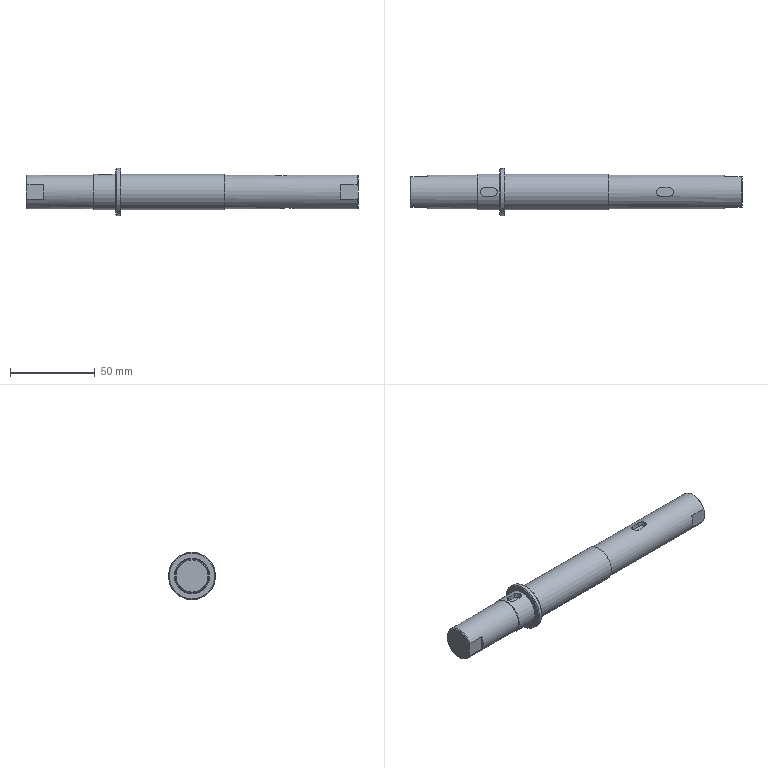Part | NX | features BREP 1 | 1 solid | 43 faces | box 196 x 28 x 28 mm | volume 62604 mm3 | plane 23 | cylinder 13 | cone 7 | commonest cylinder face diameters 5 x4 6.8 x4 20 x2 21 x2 28 x1
STEP:
#1=CARTESIAN_POINT('',(55.5,0.,14.));
#2=VERTEX_POINT('',#1);
#3=CARTESIAN_POINT('',(55.5,0.,0.));
#4=DIRECTION('',(-1.,0.,0.));
#5=DIRECTION('',(0.,0.,1.));
#6=AXIS2_PLACEMENT_3D('',#3,#4,#5);
#7=CIRCLE('',#6,14.);
#8=EDGE_CURVE('',#2,#2,#7,.T.);
#9=ORIENTED_EDGE('',*,*,#8,.F.);
#10=EDGE_LOOP('',(#9));
#11=FACE_BOUND('',#10,.T.);
#12=CARTESIAN_POINT('',(56.,0.,13.5));
#13=VERTEX_POINT('',#12);
#14=CARTESIAN_POINT('',(56.,0.,0.));
#15=DIRECTION('',(1.,0.,0.));
#16=DIRECTION('',(0.,0.,1.));
#17=AXIS2_PLACEMENT_3D('',#14,#15,#16);
#18=CIRCLE('',#17,13.5);
#19=EDGE_CURVE('',#13,#13,#18,.T.);
#20=ORIENTED_EDGE('',*,*,#19,.F.);
#21=EDGE_LOOP('',(#20));
#22=FACE_BOUND('',#21,.T.);
#23=CARTESIAN_POINT('',(55.5,0.,0.));
#24=DIRECTION('',(-1.,0.,0.));
#25=DIRECTION('',(0.,0.,1.));
#26=AXIS2_PLACEMENT_3D('',#23,#24,#25);
#27=CONICAL_SURFACE('',#26,14.,0.7854);
#28=ADVANCED_FACE('',(#11,#22),#27,.T.);
#29=CARTESIAN_POINT('',(53.5,0.,-14.));
#30=VERTEX_POINT('',#29);
#31=CARTESIAN_POINT('',(53.5,0.,0.));
#32=DIRECTION('',(1.,0.,0.));
#33=DIRECTION('',(0.,0.,-1.));
#34=AXIS2_PLACEMENT_3D('',#31,#32,#33);
#35=CIRCLE('',#34,14.);
#36=EDGE_CURVE('',#30,#30,#35,.T.);
#37=ORIENTED_EDGE('',*,*,#36,.F.);
#38=EDGE_LOOP('',(#37));
#39=FACE_BOUND('',#38,.T.);
#40=CARTESIAN_POINT('',(53.,0.,-13.5));
#41=VERTEX_POINT('',#40);
#42=CARTESIAN_POINT('',(53.,0.,0.));
#43=DIRECTION('',(-1.,0.,0.));
#44=DIRECTION('',(0.,0.,-1.));
#45=AXIS2_PLACEMENT_3D('',#42,#43,#44);
#46=CIRCLE('',#45,13.5);
#47=EDGE_CURVE('',#41,#41,#46,.T.);
#48=ORIENTED_EDGE('',*,*,#47,.F.);
#49=EDGE_LOOP('',(#48));
#50=FACE_BOUND('',#49,.T.);
#51=CARTESIAN_POINT('',(53.,0.,0.));
#52=DIRECTION('',(1.,0.,0.));
#53=DIRECTION('',(0.,0.,-1.));
#54=AXIS2_PLACEMENT_3D('',#51,#52,#53);
#55=CONICAL_SURFACE('',#54,13.5,0.7854);
#56=ADVANCED_FACE('',(#39,#50),#55,.T.);
#57=CARTESIAN_POINT('',(196.,0.,5.4));
#58=VERTEX_POINT('',#57);
#59=CARTESIAN_POINT('',(196.,0.,0.));
#60=DIRECTION('',(-1.,0.,0.));
#61=DIRECTION('',(0.,0.,1.));
#62=AXIS2_PLACEMENT_3D('',#59,#60,#61);
#63=CIRCLE('',#62,5.4);
#64=EDGE_CURVE('',#58,#58,#63,.T.);
#65=ORIENTED_EDGE('',*,*,#64,.F.);
#66=EDGE_LOOP('',(#65));
#67=FACE_BOUND('',#66,.T.);
#68=CARTESIAN_POINT('',(194.,0.,3.4));
#69=VERTEX_POINT('',#68);
#70=CARTESIAN_POINT('',(194.,0.,0.));
#71=DIRECTION('',(1.,0.,0.));
#72=DIRECTION('',(0.,0.,1.));
#73=AXIS2_PLACEMENT_3D('',#70,#71,#72);
#74=CIRCLE('',#73,3.4);
#75=EDGE_CURVE('',#69,#69,#74,.T.);
#76=ORIENTED_EDGE('',*,*,#75,.F.);
#77=EDGE_LOOP('',(#76));
#78=FACE_BOUND('',#77,.T.);
#79=CARTESIAN_POINT('',(194.,0.,0.));
#80=DIRECTION('',(1.,0.,0.));
#81=DIRECTION('',(0.,0.,-1.));
#82=AXIS2_PLACEMENT_3D('',#79,#80,#81);
#83=CONICAL_SURFACE('',#82,3.4,0.7854);
#84=ADVANCED_FACE('',(#67,#78),#83,.F.);
#85=CARTESIAN_POINT('',(196.,9.,3.041));
#86=VERTEX_POINT('',#85);
#87=CARTESIAN_POINT('',(196.,-9.,3.041));
#88=VERTEX_POINT('',#87);
#89=CARTESIAN_POINT('',(196.,0.,0.));
#90=DIRECTION('',(1.,0.,0.));
#91=DIRECTION('',(0.,0.,1.));
#92=AXIS2_PLACEMENT_3D('',#89,#90,#91);
#93=CIRCLE('',#92,9.5);
#94=EDGE_CURVE('',#86,#88,#93,.T.);
#95=ORIENTED_EDGE('',*,*,#94,.F.);
#96=CARTESIAN_POINT('',(195.5,9.,4.359));
#97=VERTEX_POINT('',#96);
#98=CARTESIAN_POINT('',(195.5,9.,4.359));
#99=CARTESIAN_POINT('',(195.688,9.,3.928));
#100=CARTESIAN_POINT('',(195.857,9.,3.489));
#101=CARTESIAN_POINT('',(196.,9.,3.041));
#102=B_SPLINE_CURVE_WITH_KNOTS('',3,(#98,#99,#100,#101),.UNSPECIFIED.,.F.,.F.,(4,4),(0.,1.),.PIECEWISE_BEZIER_KNOTS.);
#103=EDGE_CURVE('',#97,#86,#102,.T.);
#104=ORIENTED_EDGE('',*,*,#103,.F.);
#105=CARTESIAN_POINT('',(195.5,-9.,4.359));
#106=VERTEX_POINT('',#105);
#107=CARTESIAN_POINT('',(195.5,0.,0.));
#108=DIRECTION('',(-1.,0.,0.));
#109=DIRECTION('',(0.,0.,1.));
#110=AXIS2_PLACEMENT_3D('',#107,#108,#109);
#111=CIRCLE('',#110,10.);
#112=EDGE_CURVE('',#106,#97,#111,.T.);
#113=ORIENTED_EDGE('',*,*,#112,.F.);
#114=CARTESIAN_POINT('',(196.,-9.,3.041));
#115=CARTESIAN_POINT('',(195.857,-9.,3.489));
#116=CARTESIAN_POINT('',(195.688,-9.,3.928));
#117=CARTESIAN_POINT('',(195.5,-9.,4.359));
#118=B_SPLINE_CURVE_WITH_KNOTS('',3,(#114,#115,#116,#117),.UNSPECIFIED.,.F.,.F.,(4,4),(0.,1.),.PIECEWISE_BEZIER_KNOTS.);
#119=EDGE_CURVE('',#88,#106,#118,.T.);
#120=ORIENTED_EDGE('',*,*,#119,.F.);
#121=EDGE_LOOP('',(#95,#104,#113,#120));
#122=FACE_BOUND('',#121,.T.);
#123=CARTESIAN_POINT('',(195.5,0.,0.));
#124=DIRECTION('',(-1.,0.,0.));
#125=DIRECTION('',(0.,0.,1.));
#126=AXIS2_PLACEMENT_3D('',#123,#124,#125);
#127=CONICAL_SURFACE('',#126,10.,0.7854);
#128=ADVANCED_FACE('',(#122),#127,.T.);
#129=CARTESIAN_POINT('',(0.,9.,-3.041));
#130=VERTEX_POINT('',#129);
#131=CARTESIAN_POINT('',(0.,-9.,-3.041));
#132=VERTEX_POINT('',#131);
#133=CARTESIAN_POINT('',(0.,0.,0.));
#134=DIRECTION('',(-1.,0.,0.));
#135=DIRECTION('',(0.,0.,-1.));
#136=AXIS2_PLACEMENT_3D('',#133,#134,#135);
#137=CIRCLE('',#136,9.5);
#138=EDGE_CURVE('',#130,#132,#137,.T.);
#139=ORIENTED_EDGE('',*,*,#138,.F.);
#140=CARTESIAN_POINT('',(0.5,9.,-4.359));
#141=VERTEX_POINT('',#140);
#142=CARTESIAN_POINT('',(0.5,9.,-4.359));
#143=CARTESIAN_POINT('',(0.3123,9.,-3.928));
#144=CARTESIAN_POINT('',(0.1432,9.,-3.489));
#145=CARTESIAN_POINT('',(0.,9.,-3.041));
#146=B_SPLINE_CURVE_WITH_KNOTS('',3,(#142,#143,#144,#145),.UNSPECIFIED.,.F.,.F.,(4,4),(0.,1.),.PIECEWISE_BEZIER_KNOTS.);
#147=EDGE_CURVE('',#141,#130,#146,.T.);
#148=ORIENTED_EDGE('',*,*,#147,.F.);
#149=CARTESIAN_POINT('',(0.5,-9.,-4.359));
#150=VERTEX_POINT('',#149);
#151=CARTESIAN_POINT('',(0.5,0.,0.));
#152=DIRECTION('',(1.,0.,0.));
#153=DIRECTION('',(0.,0.,-1.));
#154=AXIS2_PLACEMENT_3D('',#151,#152,#153);
#155=CIRCLE('',#154,10.);
#156=EDGE_CURVE('',#150,#141,#155,.T.);
#157=ORIENTED_EDGE('',*,*,#156,.F.);
#158=CARTESIAN_POINT('',(0.,-9.,-3.041));
#159=CARTESIAN_POINT('',(0.1432,-9.,-3.489));
#160=CARTESIAN_POINT('',(0.3123,-9.,-3.928));
#161=CARTESIAN_POINT('',(0.5,-9.,-4.359));
#162=B_SPLINE_CURVE_WITH_KNOTS('',3,(#158,#159,#160,#161),.UNSPECIFIED.,.F.,.F.,(4,4),(0.,1.),.PIECEWISE_BEZIER_KNOTS.);
#163=EDGE_CURVE('',#132,#150,#162,.T.);
#164=ORIENTED_EDGE('',*,*,#163,.F.);
#165=EDGE_LOOP('',(#139,#148,#157,#164));
#166=FACE_BOUND('',#165,.T.);
#167=CARTESIAN_POINT('',(0.,0.,0.));
#168=DIRECTION('',(1.,0.,0.));
#169=DIRECTION('',(0.,0.,-1.));
#170=AXIS2_PLACEMENT_3D('',#167,#168,#169);
#171=CONICAL_SURFACE('',#170,9.5,0.7854);
#172=ADVANCED_FACE('',(#166),#171,.T.);
#173=CARTESIAN_POINT('',(117.,0.,-10.));
#174=VERTEX_POINT('',#173);
#175=CARTESIAN_POINT('',(117.,0.,0.));
#176=DIRECTION('',(1.,0.,0.));
#177=DIRECTION('',(0.,0.,-1.));
#178=AXIS2_PLACEMENT_3D('',#175,#176,#177);
#179=CIRCLE('',#178,10.);
#180=EDGE_CURVE('',#174,#174,#179,.T.);
#181=ORIENTED_EDGE('',*,*,#180,.T.);
#182=EDGE_LOOP('',(#181));
#183=FACE_BOUND('',#182,.T.);
#184=CARTESIAN_POINT('',(153.,-2.5,9.682));
#185=VERTEX_POINT('',#184);
#186=CARTESIAN_POINT('',(153.,2.5,9.682));
#187=VERTEX_POINT('',#186);
#188=CARTESIAN_POINT('',(153.,-2.5,9.682));
#189=CARTESIAN_POINT('',(153.663,-2.5,9.682));
#190=CARTESIAN_POINT('',(154.954,-1.958,9.844));
#191=CARTESIAN_POINT('',(155.773,-0.003505,10.078));
#192=CARTESIAN_POINT('',(154.955,1.959,9.844));
#193=CARTESIAN_POINT('',(153.663,2.5,9.682));
#194=CARTESIAN_POINT('',(153.,2.5,9.682));
#195=B_SPLINE_CURVE_WITH_KNOTS('',3,(#188,#189,#190,#191,#192,#193,#194),.UNSPECIFIED.,.F.,.F.,(4,1,1,1,4),(0.,0.001961,0.003922,0.005884,0.007845),.UNSPECIFIED.);
#196=EDGE_CURVE('',#185,#187,#195,.T.);
#197=ORIENTED_EDGE('',*,*,#196,.F.);
#198=CARTESIAN_POINT('',(148.,-2.5,9.682));
#199=VERTEX_POINT('',#198);
#200=CARTESIAN_POINT('',(0.,-2.5,9.682));
#201=DIRECTION('',(-1.,0.,0.));
#202=VECTOR('',#201,1000.);
#203=LINE('',#200,#202);
#204=EDGE_CURVE('',#185,#199,#203,.T.);
#205=ORIENTED_EDGE('',*,*,#204,.T.);
#206=CARTESIAN_POINT('',(148.,2.5,9.682));
#207=VERTEX_POINT('',#206);
#208=CARTESIAN_POINT('',(148.,-2.5,9.682));
#209=CARTESIAN_POINT('',(147.337,-2.5,9.682));
#210=CARTESIAN_POINT('',(146.046,-1.958,9.844));
#211=CARTESIAN_POINT('',(145.227,-0.003505,10.078));
#212=CARTESIAN_POINT('',(146.045,1.959,9.844));
#213=CARTESIAN_POINT('',(147.337,2.5,9.682));
#214=CARTESIAN_POINT('',(148.,2.5,9.682));
#215=B_SPLINE_CURVE_WITH_KNOTS('',3,(#208,#209,#210,#211,#212,#213,#214),.UNSPECIFIED.,.F.,.F.,(4,1,1,1,4),(0.,0.001961,0.003922,0.005884,0.007845),.UNSPECIFIED.);
#216=EDGE_CURVE('',#199,#207,#215,.T.);
#217=ORIENTED_EDGE('',*,*,#216,.T.);
#218=CARTESIAN_POINT('',(0.,2.5,9.682));
#219=DIRECTION('',(-1.,0.,0.));
#220=VECTOR('',#219,1000.);
#221=LINE('',#218,#220);
#222=EDGE_CURVE('',#187,#207,#221,.T.);
#223=ORIENTED_EDGE('',*,*,#222,.F.);
#224=EDGE_LOOP('',(#197,#205,#217,#223));
#225=FACE_BOUND('',#224,.T.);
#226=ORIENTED_EDGE('',*,*,#112,.T.);
#227=CARTESIAN_POINT('',(185.5,9.,4.359));
#228=VERTEX_POINT('',#227);
#229=CARTESIAN_POINT('',(185.5,9.,4.359));
#230=DIRECTION('',(1.,0.,0.));
#231=VECTOR('',#230,1000.);
#232=LINE('',#229,#231);
#233=EDGE_CURVE('',#228,#97,#232,.T.);
#234=ORIENTED_EDGE('',*,*,#233,.F.);
#235=CARTESIAN_POINT('',(185.5,9.,-4.359));
#236=VERTEX_POINT('',#235);
#237=CARTESIAN_POINT('',(185.5,0.,0.));
#238=DIRECTION('',(1.,0.,0.));
#239=DIRECTION('',(0.,0.,-1.));
#240=AXIS2_PLACEMENT_3D('',#237,#238,#239);
#241=CIRCLE('',#240,10.);
#242=EDGE_CURVE('',#236,#228,#241,.T.);
#243=ORIENTED_EDGE('',*,*,#242,.F.);
#244=CARTESIAN_POINT('',(195.5,9.,-4.359));
#245=VERTEX_POINT('',#244);
#246=CARTESIAN_POINT('',(185.5,9.,-4.359));
#247=DIRECTION('',(1.,0.,0.));
#248=VECTOR('',#247,1000.);
#249=LINE('',#246,#248);
#250=EDGE_CURVE('',#236,#245,#249,.T.);
#251=ORIENTED_EDGE('',*,*,#250,.T.);
#252=CARTESIAN_POINT('',(195.5,-9.,-4.359));
#253=VERTEX_POINT('',#252);
#254=CARTESIAN_POINT('',(195.5,0.,0.));
#255=DIRECTION('',(-1.,0.,0.));
#256=DIRECTION('',(0.,0.,1.));
#257=AXIS2_PLACEMENT_3D('',#254,#255,#256);
#258=CIRCLE('',#257,10.);
#259=EDGE_CURVE('',#245,#253,#258,.T.);
#260=ORIENTED_EDGE('',*,*,#259,.T.);
#261=CARTESIAN_POINT('',(185.5,-9.,-4.359));
#262=VERTEX_POINT('',#261);
#263=CARTESIAN_POINT('',(185.5,-9.,-4.359));
#264=DIRECTION('',(1.,0.,0.));
#265=VECTOR('',#264,1000.);
#266=LINE('',#263,#265);
#267=EDGE_CURVE('',#253,#262,#266,.F.);
#268=ORIENTED_EDGE('',*,*,#267,.T.);
#269=CARTESIAN_POINT('',(185.5,-9.,4.359));
#270=VERTEX_POINT('',#269);
#271=CARTESIAN_POINT('',(185.5,0.,0.));
#272=DIRECTION('',(1.,0.,0.));
#273=DIRECTION('',(0.,0.,-1.));
#274=AXIS2_PLACEMENT_3D('',#271,#272,#273);
#275=CIRCLE('',#274,10.);
#276=EDGE_CURVE('',#270,#262,#275,.T.);
#277=ORIENTED_EDGE('',*,*,#276,.F.);
#278=CARTESIAN_POINT('',(185.5,-9.,4.359));
#279=DIRECTION('',(1.,0.,0.));
#280=VECTOR('',#279,1000.);
#281=LINE('',#278,#280);
#282=EDGE_CURVE('',#106,#270,#281,.F.);
#283=ORIENTED_EDGE('',*,*,#282,.F.);
#284=EDGE_LOOP('',(#226,#234,#243,#251,#260,#268,#277,#283));
#285=FACE_BOUND('',#284,.T.);
#286=CARTESIAN_POINT('',(149.192,0.,-10.));
#287=VERTEX_POINT('',#286);
#288=CARTESIAN_POINT('',(149.694,-1.596,-9.901));
#289=CARTESIAN_POINT('',(148.941,0.0002752,-10.05));
#290=CARTESIAN_POINT('',(149.693,1.595,-9.901));
#291=CARTESIAN_POINT('',(151.021,2.554,-9.677));
#292=CARTESIAN_POINT('',(152.529,3.162,-9.492));
#293=CARTESIAN_POINT('',(154.665,3.539,-9.349));
#294=CARTESIAN_POINT('',(156.939,3.204,-9.507));
#295=CARTESIAN_POINT('',(158.514,1.646,-9.901));
#296=CARTESIAN_POINT('',(158.953,0.0115,-10.049));
#297=CARTESIAN_POINT('',(158.524,-1.631,-9.904));
#298=CARTESIAN_POINT('',(156.947,-3.202,-9.508));
#299=CARTESIAN_POINT('',(154.68,-3.539,-9.348));
#300=CARTESIAN_POINT('',(152.535,-3.164,-9.491));
#301=CARTESIAN_POINT('',(151.021,-2.554,-9.677));
#302=CARTESIAN_POINT('',(149.694,-1.596,-9.901));
#303=CARTESIAN_POINT('',(148.941,0.0002752,-10.05));
#304=CARTESIAN_POINT('',(149.693,1.595,-9.901));
#305=B_SPLINE_CURVE_WITH_KNOTS('',3,(#288,#289,#290,#291,#292,#293,#294,#295,#296,#297,#298,#299,#300,#301,#302,#303,#304),.UNSPECIFIED.,.T.,.F.,(1,1,1,1,1,1,1,1,1,1,1,1,1,1,1,1,1,1,1,1,1),(-0.004908,-0.003272,-0.001636,0.,0.001636,0.003272,0.004908,0.006544,0.009815,0.01145,0.01309,0.01472,0.01636,0.01963,0.02127,0.0229,0.02454,0.02617,0.02781,0.02945,0.03108),.UNSPECIFIED.);
#306=EDGE_CURVE('',#287,#287,#305,.T.);
#307=ORIENTED_EDGE('',*,*,#306,.F.);
#308=EDGE_LOOP('',(#307));
#309=FACE_BOUND('',#308,.T.);
#310=CARTESIAN_POINT('',(0.,0.,0.));
#311=DIRECTION('',(-1.,0.,0.));
#312=DIRECTION('',(0.,0.,1.));
#313=AXIS2_PLACEMENT_3D('',#310,#311,#312);
#314=CYLINDRICAL_SURFACE('',#313,10.);
#315=ADVANCED_FACE('',(#183,#225,#285,#309),#314,.T.);
#316=ORIENTED_EDGE('',*,*,#306,.T.);
#317=EDGE_LOOP('',(#316));
#318=FACE_BOUND('',#317,.T.);
#319=CARTESIAN_POINT('',(164.,-3.4,0.));
#320=VERTEX_POINT('',#319);
#321=CARTESIAN_POINT('',(165.408,0.,-3.4));
#322=VERTEX_POINT('',#321);
#323=CARTESIAN_POINT('',(164.,-3.4,0.));
#324=CARTESIAN_POINT('',(164.825,-3.4,-1.992));
#325=CARTESIAN_POINT('',(165.408,-1.992,-3.4));
#326=CARTESIAN_POINT('',(165.408,0.,-3.4));
#327=(BOUNDED_CURVE()B_SPLINE_CURVE(3,(#323,#324,#325,#326),.UNSPECIFIED.,.F.,.F.)B_SPLINE_CURVE_WITH_KNOTS((4,4),(0.,1.),.PIECEWISE_BEZIER_KNOTS.)CURVE()GEOMETRIC_REPRESENTATION_ITEM()RATIONAL_B_SPLINE_CURVE((1.,0.8047,0.8047,1.))REPRESENTATION_ITEM(''));
#328=EDGE_CURVE('',#320,#322,#327,.T.);
#329=ORIENTED_EDGE('',*,*,#328,.T.);
#330=CARTESIAN_POINT('',(164.,3.4,0.));
#331=VERTEX_POINT('',#330);
#332=CARTESIAN_POINT('',(165.408,0.,-3.4));
#333=CARTESIAN_POINT('',(165.408,1.992,-3.4));
#334=CARTESIAN_POINT('',(164.825,3.4,-1.992));
#335=CARTESIAN_POINT('',(164.,3.4,0.));
#336=(BOUNDED_CURVE()B_SPLINE_CURVE(3,(#332,#333,#334,#335),.UNSPECIFIED.,.F.,.F.)B_SPLINE_CURVE_WITH_KNOTS((4,4),(0.,1.),.PIECEWISE_BEZIER_KNOTS.)CURVE()GEOMETRIC_REPRESENTATION_ITEM()RATIONAL_B_SPLINE_CURVE((1.,0.8047,0.8047,1.))REPRESENTATION_ITEM(''));
#337=EDGE_CURVE('',#322,#331,#336,.T.);
#338=ORIENTED_EDGE('',*,*,#337,.T.);
#339=CARTESIAN_POINT('',(163.,3.375,-0.4142));
#340=VERTEX_POINT('',#339);
#341=CARTESIAN_POINT('',(164.,3.4,0.));
#342=CARTESIAN_POINT('',(163.666,3.4,-0.1385));
#343=CARTESIAN_POINT('',(163.332,3.392,-0.2767));
#344=CARTESIAN_POINT('',(163.,3.375,-0.4142));
#345=(BOUNDED_CURVE()B_SPLINE_CURVE(3,(#341,#342,#343,#344),.UNSPECIFIED.,.F.,.F.)B_SPLINE_CURVE_WITH_KNOTS((4,4),(0.,1.),.PIECEWISE_BEZIER_KNOTS.)CURVE()GEOMETRIC_REPRESENTATION_ITEM()RATIONAL_B_SPLINE_CURVE((1.,0.9988,0.9988,1.))REPRESENTATION_ITEM(''));
#346=EDGE_CURVE('',#331,#340,#345,.T.);
#347=ORIENTED_EDGE('',*,*,#346,.T.);
#348=CARTESIAN_POINT('',(163.,2.394,2.414));
#349=VERTEX_POINT('',#348);
#350=CARTESIAN_POINT('',(163.,2.394,2.414));
#351=CARTESIAN_POINT('',(163.,2.941,1.647));
#352=CARTESIAN_POINT('',(163.,3.281,0.6678));
#353=CARTESIAN_POINT('',(163.,3.375,-0.4142));
#354=(BOUNDED_CURVE()B_SPLINE_CURVE(3,(#350,#351,#352,#353),.UNSPECIFIED.,.F.,.F.)B_SPLINE_CURVE_WITH_KNOTS((4,4),(0.,1.),.PIECEWISE_BEZIER_KNOTS.)CURVE()GEOMETRIC_REPRESENTATION_ITEM()RATIONAL_B_SPLINE_CURVE((1.,0.9632,0.9632,1.))REPRESENTATION_ITEM(''));
#355=EDGE_CURVE('',#349,#340,#354,.T.);
#356=ORIENTED_EDGE('',*,*,#355,.F.);
#357=CARTESIAN_POINT('',(163.,2.394,2.414));
#358=CARTESIAN_POINT('',(163.268,3.047,1.767));
#359=CARTESIAN_POINT('',(163.619,3.4,0.9189));
#360=CARTESIAN_POINT('',(164.,3.4,0.));
#361=(BOUNDED_CURVE()B_SPLINE_CURVE(3,(#357,#358,#359,#360),.UNSPECIFIED.,.F.,.F.)B_SPLINE_CURVE_WITH_KNOTS((4,4),(0.,1.),.PIECEWISE_BEZIER_KNOTS.)CURVE()GEOMETRIC_REPRESENTATION_ITEM()RATIONAL_B_SPLINE_CURVE((1.,0.9487,0.9487,1.))REPRESENTATION_ITEM(''));
#362=EDGE_CURVE('',#349,#331,#361,.T.);
#363=ORIENTED_EDGE('',*,*,#362,.T.);
#364=CARTESIAN_POINT('',(165.858,3.312,0.7696));
#365=VERTEX_POINT('',#364);
#366=CARTESIAN_POINT('',(164.,3.4,0.));
#367=CARTESIAN_POINT('',(164.626,3.4,0.2593));
#368=CARTESIAN_POINT('',(165.248,3.37,0.517));
#369=CARTESIAN_POINT('',(165.858,3.312,0.7696));
#370=(BOUNDED_CURVE()B_SPLINE_CURVE(3,(#366,#367,#368,#369),.UNSPECIFIED.,.F.,.F.)B_SPLINE_CURVE_WITH_KNOTS((4,4),(0.,1.),.PIECEWISE_BEZIER_KNOTS.)CURVE()GEOMETRIC_REPRESENTATION_ITEM()RATIONAL_B_SPLINE_CURVE((1.,0.9957,0.9957,1.))REPRESENTATION_ITEM(''));
#371=EDGE_CURVE('',#331,#365,#370,.T.);
#372=ORIENTED_EDGE('',*,*,#371,.T.);
#373=CARTESIAN_POINT('',(165.858,-3.312,0.7696));
#374=VERTEX_POINT('',#373);
#375=CARTESIAN_POINT('',(165.314,0.,1.314));
#376=DIRECTION('',(0.7071,0.,0.7071));
#377=DIRECTION('',(0.7071,0.,-0.7071));
#378=AXIS2_PLACEMENT_3D('',#375,#376,#377);
#379=CIRCLE('',#378,3.4);
#380=EDGE_CURVE('',#365,#374,#379,.T.);
#381=ORIENTED_EDGE('',*,*,#380,.T.);
#382=CARTESIAN_POINT('',(165.858,-3.312,0.7696));
#383=CARTESIAN_POINT('',(165.248,-3.37,0.517));
#384=CARTESIAN_POINT('',(164.626,-3.4,0.2593));
#385=CARTESIAN_POINT('',(164.,-3.4,0.));
#386=(BOUNDED_CURVE()B_SPLINE_CURVE(3,(#382,#383,#384,#385),.UNSPECIFIED.,.F.,.F.)B_SPLINE_CURVE_WITH_KNOTS((4,4),(0.,1.),.PIECEWISE_BEZIER_KNOTS.)CURVE()GEOMETRIC_REPRESENTATION_ITEM()RATIONAL_B_SPLINE_CURVE((1.,0.9957,0.9957,1.))REPRESENTATION_ITEM(''));
#387=EDGE_CURVE('',#374,#320,#386,.T.);
#388=ORIENTED_EDGE('',*,*,#387,.T.);
#389=CARTESIAN_POINT('',(163.,-2.394,2.414));
#390=VERTEX_POINT('',#389);
#391=CARTESIAN_POINT('',(164.,-3.4,0.));
#392=CARTESIAN_POINT('',(163.619,-3.4,0.9189));
#393=CARTESIAN_POINT('',(163.268,-3.047,1.767));
#394=CARTESIAN_POINT('',(163.,-2.394,2.414));
#395=(BOUNDED_CURVE()B_SPLINE_CURVE(3,(#391,#392,#393,#394),.UNSPECIFIED.,.F.,.F.)B_SPLINE_CURVE_WITH_KNOTS((4,4),(0.,1.),.PIECEWISE_BEZIER_KNOTS.)CURVE()GEOMETRIC_REPRESENTATION_ITEM()RATIONAL_B_SPLINE_CURVE((1.,0.9487,0.9487,1.))REPRESENTATION_ITEM(''));
#396=EDGE_CURVE('',#320,#390,#395,.T.);
#397=ORIENTED_EDGE('',*,*,#396,.T.);
#398=CARTESIAN_POINT('',(163.,-3.375,-0.4142));
#399=VERTEX_POINT('',#398);
#400=CARTESIAN_POINT('',(163.,-3.375,-0.4142));
#401=CARTESIAN_POINT('',(163.,-3.281,0.6678));
#402=CARTESIAN_POINT('',(163.,-2.941,1.647));
#403=CARTESIAN_POINT('',(163.,-2.394,2.414));
#404=(BOUNDED_CURVE()B_SPLINE_CURVE(3,(#400,#401,#402,#403),.UNSPECIFIED.,.F.,.F.)B_SPLINE_CURVE_WITH_KNOTS((4,4),(0.,1.),.PIECEWISE_BEZIER_KNOTS.)CURVE()GEOMETRIC_REPRESENTATION_ITEM()RATIONAL_B_SPLINE_CURVE((1.,0.9632,0.9632,1.))REPRESENTATION_ITEM(''));
#405=EDGE_CURVE('',#399,#390,#404,.T.);
#406=ORIENTED_EDGE('',*,*,#405,.F.);
#407=CARTESIAN_POINT('',(163.,-3.375,-0.4142));
#408=CARTESIAN_POINT('',(163.332,-3.392,-0.2767));
#409=CARTESIAN_POINT('',(163.666,-3.4,-0.1385));
#410=CARTESIAN_POINT('',(164.,-3.4,0.));
#411=(BOUNDED_CURVE()B_SPLINE_CURVE(3,(#407,#408,#409,#410),.UNSPECIFIED.,.F.,.F.)B_SPLINE_CURVE_WITH_KNOTS((4,4),(0.,1.),.PIECEWISE_BEZIER_KNOTS.)CURVE()GEOMETRIC_REPRESENTATION_ITEM()RATIONAL_B_SPLINE_CURVE((1.,0.9988,0.9988,1.))REPRESENTATION_ITEM(''));
#412=EDGE_CURVE('',#399,#320,#411,.T.);
#413=ORIENTED_EDGE('',*,*,#412,.T.);
#414=EDGE_LOOP('',(#329,#338,#347,#356,#363,#372,#381,#388,#397,#406,#413));
#415=FACE_BOUND('',#414,.T.);
#416=CARTESIAN_POINT('',(165.314,0.,1.314));
#417=DIRECTION('',(-0.7071,0.,-0.7071));
#418=DIRECTION('',(-0.7071,0.,0.7071));
#419=AXIS2_PLACEMENT_3D('',#416,#417,#418);
#420=CYLINDRICAL_SURFACE('',#419,3.4);
#421=ADVANCED_FACE('',(#318,#415),#420,.F.);
#422=CARTESIAN_POINT('',(153.,2.5,7.));
#423=VERTEX_POINT('',#422);
#424=CARTESIAN_POINT('',(153.,-2.5,7.));
#425=VERTEX_POINT('',#424);
#426=CARTESIAN_POINT('',(153.,0.,7.));
#427=DIRECTION('',(0.,0.,-1.));
#428=DIRECTION('',(-1.,0.,0.));
#429=AXIS2_PLACEMENT_3D('',#426,#427,#428);
#430=CIRCLE('',#429,2.5);
#431=EDGE_CURVE('',#423,#425,#430,.T.);
#432=ORIENTED_EDGE('',*,*,#431,.T.);
#433=CARTESIAN_POINT('',(153.,-2.5,7.));
#434=DIRECTION('',(0.,0.,1.));
#435=VECTOR('',#434,1000.);
#436=LINE('',#433,#435);
#437=EDGE_CURVE('',#425,#185,#436,.T.);
#438=ORIENTED_EDGE('',*,*,#437,.T.);
#439=ORIENTED_EDGE('',*,*,#196,.T.);
#440=CARTESIAN_POINT('',(153.,2.5,7.));
#441=DIRECTION('',(0.,0.,1.));
#442=VECTOR('',#441,1000.);
#443=LINE('',#440,#442);
#444=EDGE_CURVE('',#423,#187,#443,.T.);
#445=ORIENTED_EDGE('',*,*,#444,.F.);
#446=EDGE_LOOP('',(#432,#438,#439,#445));
#447=FACE_BOUND('',#446,.T.);
#448=CARTESIAN_POINT('',(153.,0.,7.));
#449=DIRECTION('',(0.,0.,1.));
#450=DIRECTION('',(1.,0.,0.));
#451=AXIS2_PLACEMENT_3D('',#448,#449,#450);
#452=CYLINDRICAL_SURFACE('',#451,2.5);
#453=ADVANCED_FACE('',(#447),#452,.F.);
#454=ORIENTED_EDGE('',*,*,#75,.T.);
#455=EDGE_LOOP('',(#454));
#456=FACE_BOUND('',#455,.T.);
#457=CARTESIAN_POINT('',(163.227,0.,3.4));
#458=VERTEX_POINT('',#457);
#459=CARTESIAN_POINT('',(165.858,-3.312,0.7696));
#460=CARTESIAN_POINT('',(164.252,-2.939,2.375));
#461=CARTESIAN_POINT('',(163.227,-1.648,3.4));
#462=CARTESIAN_POINT('',(163.227,0.,3.4));
#463=(BOUNDED_CURVE()B_SPLINE_CURVE(3,(#459,#460,#461,#462),.UNSPECIFIED.,.F.,.F.)B_SPLINE_CURVE_WITH_KNOTS((4,4),(0.,1.),.PIECEWISE_BEZIER_KNOTS.)CURVE()GEOMETRIC_REPRESENTATION_ITEM()RATIONAL_B_SPLINE_CURVE((1.,0.8554,0.8554,1.))REPRESENTATION_ITEM(''));
#464=EDGE_CURVE('',#374,#458,#463,.T.);
#465=ORIENTED_EDGE('',*,*,#464,.T.);
#466=CARTESIAN_POINT('',(163.227,0.,3.4));
#467=CARTESIAN_POINT('',(163.227,1.648,3.4));
#468=CARTESIAN_POINT('',(164.252,2.939,2.375));
#469=CARTESIAN_POINT('',(165.858,3.312,0.7696));
#470=(BOUNDED_CURVE()B_SPLINE_CURVE(3,(#466,#467,#468,#469),.UNSPECIFIED.,.F.,.F.)B_SPLINE_CURVE_WITH_KNOTS((4,4),(0.,1.),.PIECEWISE_BEZIER_KNOTS.)CURVE()GEOMETRIC_REPRESENTATION_ITEM()RATIONAL_B_SPLINE_CURVE((1.,0.8554,0.8554,1.))REPRESENTATION_ITEM(''));
#471=EDGE_CURVE('',#458,#365,#470,.T.);
#472=ORIENTED_EDGE('',*,*,#471,.T.);
#473=ORIENTED_EDGE('',*,*,#371,.F.);
#474=ORIENTED_EDGE('',*,*,#337,.F.);
#475=ORIENTED_EDGE('',*,*,#328,.F.);
#476=ORIENTED_EDGE('',*,*,#387,.F.);
#477=EDGE_LOOP('',(#465,#472,#473,#474,#475,#476));
#478=FACE_BOUND('',#477,.T.);
#479=CARTESIAN_POINT('',(163.,0.,0.));
#480=DIRECTION('',(1.,0.,0.));
#481=DIRECTION('',(0.,0.,-1.));
#482=AXIS2_PLACEMENT_3D('',#479,#480,#481);
#483=CYLINDRICAL_SURFACE('',#482,3.4);
#484=ADVANCED_FACE('',(#456,#478),#483,.F.);
#485=CARTESIAN_POINT('',(56.,0.,10.5));
#486=VERTEX_POINT('',#485);
#487=CARTESIAN_POINT('',(56.,0.,0.));
#488=DIRECTION('',(1.,0.,0.));
#489=DIRECTION('',(0.,0.,1.));
#490=AXIS2_PLACEMENT_3D('',#487,#488,#489);
#491=CIRCLE('',#490,10.5);
#492=EDGE_CURVE('',#486,#486,#491,.T.);
#493=ORIENTED_EDGE('',*,*,#492,.T.);
#494=EDGE_LOOP('',(#493));
#495=FACE_BOUND('',#494,.T.);
#496=CARTESIAN_POINT('',(117.,0.,-10.5));
#497=VERTEX_POINT('',#496);
#498=CARTESIAN_POINT('',(117.,0.,0.));
#499=DIRECTION('',(1.,0.,0.));
#500=DIRECTION('',(0.,0.,-1.));
#501=AXIS2_PLACEMENT_3D('',#498,#499,#500);
#502=CIRCLE('',#501,10.5);
#503=EDGE_CURVE('',#497,#497,#502,.T.);
#504=ORIENTED_EDGE('',*,*,#503,.F.);
#505=EDGE_LOOP('',(#504));
#506=FACE_BOUND('',#505,.T.);
#507=CARTESIAN_POINT('',(117.,0.,0.));
#508=DIRECTION('',(-1.,0.,0.));
#509=DIRECTION('',(0.,0.,1.));
#510=AXIS2_PLACEMENT_3D('',#507,#508,#509);
#511=CYLINDRICAL_SURFACE('',#510,10.5);
#512=ADVANCED_FACE('',(#495,#506),#511,.T.);
#513=CARTESIAN_POINT('',(44.,2.5,10.198));
#514=VERTEX_POINT('',#513);
#515=CARTESIAN_POINT('',(44.,-2.5,10.198));
#516=VERTEX_POINT('',#515);
#517=CARTESIAN_POINT('',(44.,2.5,10.198));
#518=CARTESIAN_POINT('',(43.337,2.5,10.198));
#519=CARTESIAN_POINT('',(42.046,1.958,10.351));
#520=CARTESIAN_POINT('',(41.227,0.003401,10.574));
#521=CARTESIAN_POINT('',(42.045,-1.959,10.351));
#522=CARTESIAN_POINT('',(43.337,-2.5,10.198));
#523=CARTESIAN_POINT('',(44.,-2.5,10.198));
#524=B_SPLINE_CURVE_WITH_KNOTS('',3,(#517,#518,#519,#520,#521,#522,#523),.UNSPECIFIED.,.F.,.F.,(4,1,1,1,4),(0.,0.001961,0.003921,0.005882,0.007842),.UNSPECIFIED.);
#525=EDGE_CURVE('',#514,#516,#524,.T.);
#526=ORIENTED_EDGE('',*,*,#525,.T.);
#527=CARTESIAN_POINT('',(44.,-2.5,7.5));
#528=VERTEX_POINT('',#527);
#529=CARTESIAN_POINT('',(44.,-2.5,14.));
#530=DIRECTION('',(0.,0.,-1.));
#531=VECTOR('',#530,1000.);
#532=LINE('',#529,#531);
#533=EDGE_CURVE('',#516,#528,#532,.T.);
#534=ORIENTED_EDGE('',*,*,#533,.T.);
#535=CARTESIAN_POINT('',(44.,2.5,7.5));
#536=VERTEX_POINT('',#535);
#537=CARTESIAN_POINT('',(44.,0.,7.5));
#538=DIRECTION('',(0.,0.,1.));
#539=DIRECTION('',(1.,0.,0.));
#540=AXIS2_PLACEMENT_3D('',#537,#538,#539);
#541=CIRCLE('',#540,2.5);
#542=EDGE_CURVE('',#536,#528,#541,.T.);
#543=ORIENTED_EDGE('',*,*,#542,.F.);
#544=CARTESIAN_POINT('',(44.,2.5,14.));
#545=DIRECTION('',(0.,0.,-1.));
#546=VECTOR('',#545,1000.);
#547=LINE('',#544,#546);
#548=EDGE_CURVE('',#514,#536,#547,.T.);
#549=ORIENTED_EDGE('',*,*,#548,.F.);
#550=EDGE_LOOP('',(#526,#534,#543,#549));
#551=FACE_BOUND('',#550,.T.);
#552=CARTESIAN_POINT('',(44.,0.,14.));
#553=DIRECTION('',(0.,0.,-1.));
#554=DIRECTION('',(-1.,0.,0.));
#555=AXIS2_PLACEMENT_3D('',#552,#553,#554);
#556=CYLINDRICAL_SURFACE('',#555,2.5);
#557=ADVANCED_FACE('',(#551),#556,.F.);
#558=ORIENTED_EDGE('',*,*,#36,.T.);
#559=EDGE_LOOP('',(#558));
#560=FACE_BOUND('',#559,.T.);
#561=ORIENTED_EDGE('',*,*,#8,.T.);
#562=EDGE_LOOP('',(#561));
#563=FACE_BOUND('',#562,.T.);
#564=CARTESIAN_POINT('',(0.,0.,0.));
#565=DIRECTION('',(-1.,0.,0.));
#566=DIRECTION('',(0.,0.,1.));
#567=AXIS2_PLACEMENT_3D('',#564,#565,#566);
#568=CYLINDRICAL_SURFACE('',#567,14.);
#569=ADVANCED_FACE('',(#560,#563),#568,.T.);
#570=CARTESIAN_POINT('',(40.1,0.,10.5));
#571=VERTEX_POINT('',#570);
#572=CARTESIAN_POINT('',(40.1,0.,0.));
#573=DIRECTION('',(-1.,0.,0.));
#574=DIRECTION('',(0.,0.,1.));
#575=AXIS2_PLACEMENT_3D('',#572,#573,#574);
#576=CIRCLE('',#575,10.5);
#577=EDGE_CURVE('',#571,#571,#576,.T.);
#578=ORIENTED_EDGE('',*,*,#577,.F.);
#579=EDGE_LOOP('',(#578));
#580=FACE_BOUND('',#579,.T.);
#581=CARTESIAN_POINT('',(49.,-2.5,10.198));
#582=VERTEX_POINT('',#581);
#583=CARTESIAN_POINT('',(49.,2.5,10.198));
#584=VERTEX_POINT('',#583);
#585=CARTESIAN_POINT('',(49.,-2.5,10.198));
#586=CARTESIAN_POINT('',(49.663,-2.5,10.198));
#587=CARTESIAN_POINT('',(50.954,-1.958,10.351));
#588=CARTESIAN_POINT('',(51.773,-0.003401,10.574));
#589=CARTESIAN_POINT('',(50.955,1.959,10.351));
#590=CARTESIAN_POINT('',(49.663,2.5,10.198));
#591=CARTESIAN_POINT('',(49.,2.5,10.198));
#592=B_SPLINE_CURVE_WITH_KNOTS('',3,(#585,#586,#587,#588,#589,#590,#591),.UNSPECIFIED.,.F.,.F.,(4,1,1,1,4),(0.,0.001961,0.003921,0.005882,0.007842),.UNSPECIFIED.);
#593=EDGE_CURVE('',#582,#584,#592,.T.);
#594=ORIENTED_EDGE('',*,*,#593,.F.);
#595=CARTESIAN_POINT('',(0.,-2.5,10.198));
#596=DIRECTION('',(1.,0.,0.));
#597=VECTOR('',#596,1000.);
#598=LINE('',#595,#597);
#599=EDGE_CURVE('',#516,#582,#598,.T.);
#600=ORIENTED_EDGE('',*,*,#599,.F.);
#601=ORIENTED_EDGE('',*,*,#525,.F.);
#602=CARTESIAN_POINT('',(0.,2.5,10.198));
#603=DIRECTION('',(-1.,0.,0.));
#604=VECTOR('',#603,1000.);
#605=LINE('',#602,#604);
#606=EDGE_CURVE('',#584,#514,#605,.T.);
#607=ORIENTED_EDGE('',*,*,#606,.F.);
#608=EDGE_LOOP('',(#594,#600,#601,#607));
#609=FACE_BOUND('',#608,.T.);
#610=CARTESIAN_POINT('',(53.,0.,10.5));
#611=VERTEX_POINT('',#610);
#612=CARTESIAN_POINT('',(53.,0.,0.));
#613=DIRECTION('',(-1.,0.,0.));
#614=DIRECTION('',(0.,0.,1.));
#615=AXIS2_PLACEMENT_3D('',#612,#613,#614);
#616=CIRCLE('',#615,10.5);
#617=EDGE_CURVE('',#611,#611,#616,.T.);
#618=ORIENTED_EDGE('',*,*,#617,.T.);
#619=EDGE_LOOP('',(#618));
#620=FACE_BOUND('',#619,.T.);
#621=CARTESIAN_POINT('',(0.,0.,0.));
#622=DIRECTION('',(-1.,0.,0.));
#623=DIRECTION('',(0.,0.,1.));
#624=AXIS2_PLACEMENT_3D('',#621,#622,#623);
#625=CYLINDRICAL_SURFACE('',#624,10.5);
#626=ADVANCED_FACE('',(#580,#609,#620),#625,.T.);
#627=CARTESIAN_POINT('',(0.5,9.,4.359));
#628=VERTEX_POINT('',#627);
#629=CARTESIAN_POINT('',(0.5,-9.,4.359));
#630=VERTEX_POINT('',#629);
#631=CARTESIAN_POINT('',(0.5,0.,0.));
#632=DIRECTION('',(1.,0.,0.));
#633=DIRECTION('',(0.,0.,-1.));
#634=AXIS2_PLACEMENT_3D('',#631,#632,#633);
#635=CIRCLE('',#634,10.);
#636=EDGE_CURVE('',#628,#630,#635,.T.);
#637=ORIENTED_EDGE('',*,*,#636,.T.);
#638=CARTESIAN_POINT('',(10.5,-9.,4.359));
#639=VERTEX_POINT('',#638);
#640=CARTESIAN_POINT('',(10.5,-9.,4.359));
#641=DIRECTION('',(-1.,0.,0.));
#642=VECTOR('',#641,1000.);
#643=LINE('',#640,#642);
#644=EDGE_CURVE('',#639,#630,#643,.T.);
#645=ORIENTED_EDGE('',*,*,#644,.F.);
#646=CARTESIAN_POINT('',(10.5,-9.,-4.359));
#647=VERTEX_POINT('',#646);
#648=CARTESIAN_POINT('',(10.5,0.,0.));
#649=DIRECTION('',(1.,0.,0.));
#650=DIRECTION('',(0.,0.,-1.));
#651=AXIS2_PLACEMENT_3D('',#648,#649,#650);
#652=CIRCLE('',#651,10.);
#653=EDGE_CURVE('',#639,#647,#652,.T.);
#654=ORIENTED_EDGE('',*,*,#653,.T.);
#655=CARTESIAN_POINT('',(10.5,-9.,-4.359));
#656=DIRECTION('',(-1.,0.,0.));
#657=VECTOR('',#656,1000.);
#658=LINE('',#655,#657);
#659=EDGE_CURVE('',#647,#150,#658,.T.);
#660=ORIENTED_EDGE('',*,*,#659,.T.);
#661=ORIENTED_EDGE('',*,*,#156,.T.);
#662=CARTESIAN_POINT('',(10.5,9.,-4.359));
#663=VERTEX_POINT('',#662);
#664=CARTESIAN_POINT('',(10.5,9.,-4.359));
#665=DIRECTION('',(1.,0.,0.));
#666=VECTOR('',#665,1000.);
#667=LINE('',#664,#666);
#668=EDGE_CURVE('',#141,#663,#667,.T.);
#669=ORIENTED_EDGE('',*,*,#668,.T.);
#670=CARTESIAN_POINT('',(10.5,9.,4.359));
#671=VERTEX_POINT('',#670);
#672=CARTESIAN_POINT('',(10.5,0.,0.));
#673=DIRECTION('',(1.,0.,0.));
#674=DIRECTION('',(0.,0.,-1.));
#675=AXIS2_PLACEMENT_3D('',#672,#673,#674);
#676=CIRCLE('',#675,10.);
#677=EDGE_CURVE('',#663,#671,#676,.T.);
#678=ORIENTED_EDGE('',*,*,#677,.T.);
#679=CARTESIAN_POINT('',(10.5,9.,4.359));
#680=DIRECTION('',(1.,0.,0.));
#681=VECTOR('',#680,1000.);
#682=LINE('',#679,#681);
#683=EDGE_CURVE('',#628,#671,#682,.T.);
#684=ORIENTED_EDGE('',*,*,#683,.F.);
#685=EDGE_LOOP('',(#637,#645,#654,#660,#661,#669,#678,#684));
#686=FACE_BOUND('',#685,.T.);
#687=CARTESIAN_POINT('',(40.1,0.,10.));
#688=VERTEX_POINT('',#687);
#689=CARTESIAN_POINT('',(40.1,0.,0.));
#690=DIRECTION('',(-1.,0.,0.));
#691=DIRECTION('',(0.,0.,1.));
#692=AXIS2_PLACEMENT_3D('',#689,#690,#691);
#693=CIRCLE('',#692,10.);
#694=EDGE_CURVE('',#688,#688,#693,.T.);
#695=ORIENTED_EDGE('',*,*,#694,.T.);
#696=EDGE_LOOP('',(#695));
#697=FACE_BOUND('',#696,.T.);
#698=CARTESIAN_POINT('',(0.,0.,0.));
#699=DIRECTION('',(-1.,0.,0.));
#700=DIRECTION('',(0.,0.,1.));
#701=AXIS2_PLACEMENT_3D('',#698,#699,#700);
#702=CYLINDRICAL_SURFACE('',#701,10.);
#703=ADVANCED_FACE('',(#686,#697),#702,.T.);
#704=ORIENTED_EDGE('',*,*,#19,.T.);
#705=EDGE_LOOP('',(#704));
#706=FACE_BOUND('',#705,.T.);
#707=ORIENTED_EDGE('',*,*,#492,.F.);
#708=EDGE_LOOP('',(#707));
#709=FACE_BOUND('',#708,.T.);
#710=CARTESIAN_POINT('',(56.,10.,0.));
#711=DIRECTION('',(-1.,0.,0.));
#712=DIRECTION('',(0.,0.,1.));
#713=AXIS2_PLACEMENT_3D('',#710,#711,#712);
#714=PLANE('',#713);
#715=ADVANCED_FACE('',(#706,#709),#714,.F.);
#716=CARTESIAN_POINT('',(0.,-9.,3.041));
#717=VERTEX_POINT('',#716);
#718=CARTESIAN_POINT('',(0.,-9.,-4.359));
#719=DIRECTION('',(0.,0.,1.));
#720=VECTOR('',#719,1000.);
#721=LINE('',#718,#720);
#722=EDGE_CURVE('',#132,#717,#721,.T.);
#723=ORIENTED_EDGE('',*,*,#722,.T.);
#724=CARTESIAN_POINT('',(0.,9.,3.041));
#725=VERTEX_POINT('',#724);
#726=CARTESIAN_POINT('',(0.,0.,0.));
#727=DIRECTION('',(-1.,0.,0.));
#728=DIRECTION('',(0.,0.,-1.));
#729=AXIS2_PLACEMENT_3D('',#726,#727,#728);
#730=CIRCLE('',#729,9.5);
#731=EDGE_CURVE('',#717,#725,#730,.T.);
#732=ORIENTED_EDGE('',*,*,#731,.T.);
#733=CARTESIAN_POINT('',(0.,9.,-4.359));
#734=DIRECTION('',(0.,0.,-1.));
#735=VECTOR('',#734,1000.);
#736=LINE('',#733,#735);
#737=EDGE_CURVE('',#725,#130,#736,.T.);
#738=ORIENTED_EDGE('',*,*,#737,.T.);
#739=ORIENTED_EDGE('',*,*,#138,.T.);
#740=EDGE_LOOP('',(#723,#732,#738,#739));
#741=FACE_BOUND('',#740,.T.);
#742=CARTESIAN_POINT('',(0.,0.,0.));
#743=DIRECTION('',(1.,0.,0.));
#744=DIRECTION('',(0.,0.,-1.));
#745=AXIS2_PLACEMENT_3D('',#742,#743,#744);
#746=PLANE('',#745);
#747=ADVANCED_FACE('',(#741),#746,.F.);
#748=ORIENTED_EDGE('',*,*,#694,.F.);
#749=EDGE_LOOP('',(#748));
#750=FACE_BOUND('',#749,.T.);
#751=ORIENTED_EDGE('',*,*,#577,.T.);
#752=EDGE_LOOP('',(#751));
#753=FACE_BOUND('',#752,.T.);
#754=CARTESIAN_POINT('',(40.1,10.,0.));
#755=DIRECTION('',(1.,0.,0.));
#756=DIRECTION('',(0.,0.,-1.));
#757=AXIS2_PLACEMENT_3D('',#754,#755,#756);
#758=PLANE('',#757);
#759=ADVANCED_FACE('',(#750,#753),#758,.F.);
#760=ORIENTED_EDGE('',*,*,#47,.T.);
#761=EDGE_LOOP('',(#760));
#762=FACE_BOUND('',#761,.T.);
#763=ORIENTED_EDGE('',*,*,#617,.F.);
#764=EDGE_LOOP('',(#763));
#765=FACE_BOUND('',#764,.T.);
#766=CARTESIAN_POINT('',(53.,14.,0.));
#767=DIRECTION('',(1.,0.,0.));
#768=DIRECTION('',(0.,0.,-1.));
#769=AXIS2_PLACEMENT_3D('',#766,#767,#768);
#770=PLANE('',#769);
#771=ADVANCED_FACE('',(#762,#765),#770,.F.);
#772=CARTESIAN_POINT('',(49.,-2.5,7.5));
#773=VERTEX_POINT('',#772);
#774=CARTESIAN_POINT('',(49.,-2.5,14.));
#775=DIRECTION('',(0.,0.,-1.));
#776=VECTOR('',#775,1000.);
#777=LINE('',#774,#776);
#778=EDGE_CURVE('',#582,#773,#777,.T.);
#779=ORIENTED_EDGE('',*,*,#778,.F.);
#780=ORIENTED_EDGE('',*,*,#593,.T.);
#781=CARTESIAN_POINT('',(49.,2.5,7.5));
#782=VERTEX_POINT('',#781);
#783=CARTESIAN_POINT('',(49.,2.5,14.));
#784=DIRECTION('',(0.,0.,-1.));
#785=VECTOR('',#784,1000.);
#786=LINE('',#783,#785);
#787=EDGE_CURVE('',#584,#782,#786,.T.);
#788=ORIENTED_EDGE('',*,*,#787,.T.);
#789=CARTESIAN_POINT('',(49.,0.,7.5));
#790=DIRECTION('',(0.,0.,1.));
#791=DIRECTION('',(1.,0.,0.));
#792=AXIS2_PLACEMENT_3D('',#789,#790,#791);
#793=CIRCLE('',#792,2.5);
#794=EDGE_CURVE('',#773,#782,#793,.T.);
#795=ORIENTED_EDGE('',*,*,#794,.F.);
#796=EDGE_LOOP('',(#779,#780,#788,#795));
#797=FACE_BOUND('',#796,.T.);
#798=CARTESIAN_POINT('',(49.,0.,14.));
#799=DIRECTION('',(0.,0.,-1.));
#800=DIRECTION('',(-1.,0.,0.));
#801=AXIS2_PLACEMENT_3D('',#798,#799,#800);
#802=CYLINDRICAL_SURFACE('',#801,2.5);
#803=ADVANCED_FACE('',(#797),#802,.F.);
#804=ORIENTED_EDGE('',*,*,#606,.T.);
#805=ORIENTED_EDGE('',*,*,#548,.T.);
#806=CARTESIAN_POINT('',(44.,2.5,7.5));
#807=DIRECTION('',(-1.,0.,0.));
#808=VECTOR('',#807,1000.);
#809=LINE('',#806,#808);
#810=EDGE_CURVE('',#782,#536,#809,.T.);
#811=ORIENTED_EDGE('',*,*,#810,.F.);
#812=ORIENTED_EDGE('',*,*,#787,.F.);
#813=EDGE_LOOP('',(#804,#805,#811,#812));
#814=FACE_BOUND('',#813,.T.);
#815=CARTESIAN_POINT('',(44.,2.5,14.));
#816=DIRECTION('',(0.,-1.,0.));
#817=DIRECTION('',(1.,0.,0.));
#818=AXIS2_PLACEMENT_3D('',#815,#816,#817);
#819=PLANE('',#818);
#820=ADVANCED_FACE('',(#814),#819,.T.);
#821=ORIENTED_EDGE('',*,*,#599,.T.);
#822=ORIENTED_EDGE('',*,*,#778,.T.);
#823=CARTESIAN_POINT('',(44.,-2.5,7.5));
#824=DIRECTION('',(1.,0.,0.));
#825=VECTOR('',#824,1000.);
#826=LINE('',#823,#825);
#827=EDGE_CURVE('',#528,#773,#826,.T.);
#828=ORIENTED_EDGE('',*,*,#827,.F.);
#829=ORIENTED_EDGE('',*,*,#533,.F.);
#830=EDGE_LOOP('',(#821,#822,#828,#829));
#831=FACE_BOUND('',#830,.T.);
#832=CARTESIAN_POINT('',(44.,-2.5,14.));
#833=DIRECTION('',(0.,1.,0.));
#834=DIRECTION('',(-1.,0.,0.));
#835=AXIS2_PLACEMENT_3D('',#832,#833,#834);
#836=PLANE('',#835);
#837=ADVANCED_FACE('',(#831),#836,.T.);
#838=ORIENTED_EDGE('',*,*,#794,.T.);
#839=ORIENTED_EDGE('',*,*,#810,.T.);
#840=ORIENTED_EDGE('',*,*,#542,.T.);
#841=ORIENTED_EDGE('',*,*,#827,.T.);
#842=EDGE_LOOP('',(#838,#839,#840,#841));
#843=FACE_BOUND('',#842,.T.);
#844=CARTESIAN_POINT('',(49.,0.,7.5));
#845=DIRECTION('',(0.,0.,1.));
#846=DIRECTION('',(1.,0.,0.));
#847=AXIS2_PLACEMENT_3D('',#844,#845,#846);
#848=PLANE('',#847);
#849=ADVANCED_FACE('',(#843),#848,.T.);
#850=ORIENTED_EDGE('',*,*,#737,.F.);
#851=CARTESIAN_POINT('',(0.,9.,3.041));
#852=CARTESIAN_POINT('',(0.1432,9.,3.489));
#853=CARTESIAN_POINT('',(0.3123,9.,3.928));
#854=CARTESIAN_POINT('',(0.5,9.,4.359));
#855=B_SPLINE_CURVE_WITH_KNOTS('',3,(#851,#852,#853,#854),.UNSPECIFIED.,.F.,.F.,(4,4),(0.,1.),.PIECEWISE_BEZIER_KNOTS.);
#856=EDGE_CURVE('',#725,#628,#855,.T.);
#857=ORIENTED_EDGE('',*,*,#856,.T.);
#858=ORIENTED_EDGE('',*,*,#683,.T.);
#859=CARTESIAN_POINT('',(10.5,9.,-4.359));
#860=DIRECTION('',(0.,0.,-1.));
#861=VECTOR('',#860,1000.);
#862=LINE('',#859,#861);
#863=EDGE_CURVE('',#671,#663,#862,.T.);
#864=ORIENTED_EDGE('',*,*,#863,.T.);
#865=ORIENTED_EDGE('',*,*,#668,.F.);
#866=ORIENTED_EDGE('',*,*,#147,.T.);
#867=EDGE_LOOP('',(#850,#857,#858,#864,#865,#866));
#868=FACE_BOUND('',#867,.T.);
#869=CARTESIAN_POINT('',(10.5,9.,-4.359));
#870=DIRECTION('',(0.,1.,0.));
#871=DIRECTION('',(0.,0.,1.));
#872=AXIS2_PLACEMENT_3D('',#869,#870,#871);
#873=PLANE('',#872);
#874=ADVANCED_FACE('',(#868),#873,.T.);
#875=ORIENTED_EDGE('',*,*,#677,.F.);
#876=ORIENTED_EDGE('',*,*,#863,.F.);
#877=EDGE_LOOP('',(#875,#876));
#878=FACE_BOUND('',#877,.T.);
#879=CARTESIAN_POINT('',(10.5,0.,0.));
#880=DIRECTION('',(-1.,0.,0.));
#881=DIRECTION('',(0.,0.,-1.));
#882=AXIS2_PLACEMENT_3D('',#879,#880,#881);
#883=PLANE('',#882);
#884=ADVANCED_FACE('',(#878),#883,.T.);
#885=ORIENTED_EDGE('',*,*,#644,.T.);
#886=CARTESIAN_POINT('',(0.5,-9.,4.359));
#887=CARTESIAN_POINT('',(0.3123,-9.,3.928));
#888=CARTESIAN_POINT('',(0.1432,-9.,3.489));
#889=CARTESIAN_POINT('',(0.,-9.,3.041));
#890=B_SPLINE_CURVE_WITH_KNOTS('',3,(#886,#887,#888,#889),.UNSPECIFIED.,.F.,.F.,(4,4),(0.,1.),.PIECEWISE_BEZIER_KNOTS.);
#891=EDGE_CURVE('',#630,#717,#890,.T.);
#892=ORIENTED_EDGE('',*,*,#891,.T.);
#893=ORIENTED_EDGE('',*,*,#722,.F.);
#894=ORIENTED_EDGE('',*,*,#163,.T.);
#895=ORIENTED_EDGE('',*,*,#659,.F.);
#896=CARTESIAN_POINT('',(10.5,-9.,-4.359));
#897=DIRECTION('',(0.,0.,1.));
#898=VECTOR('',#897,1000.);
#899=LINE('',#896,#898);
#900=EDGE_CURVE('',#647,#639,#899,.T.);
#901=ORIENTED_EDGE('',*,*,#900,.T.);
#902=EDGE_LOOP('',(#885,#892,#893,#894,#895,#901));
#903=FACE_BOUND('',#902,.T.);
#904=CARTESIAN_POINT('',(10.5,-9.,-4.359));
#905=DIRECTION('',(0.,-1.,0.));
#906=DIRECTION('',(0.,0.,-1.));
#907=AXIS2_PLACEMENT_3D('',#904,#905,#906);
#908=PLANE('',#907);
#909=ADVANCED_FACE('',(#903),#908,.T.);
#910=ORIENTED_EDGE('',*,*,#653,.F.);
#911=ORIENTED_EDGE('',*,*,#900,.F.);
#912=EDGE_LOOP('',(#910,#911));
#913=FACE_BOUND('',#912,.T.);
#914=CARTESIAN_POINT('',(10.5,0.,0.));
#915=DIRECTION('',(-1.,0.,0.));
#916=DIRECTION('',(0.,0.,-1.));
#917=AXIS2_PLACEMENT_3D('',#914,#915,#916);
#918=PLANE('',#917);
#919=ADVANCED_FACE('',(#913),#918,.T.);
#920=ORIENTED_EDGE('',*,*,#503,.T.);
#921=EDGE_LOOP('',(#920));
#922=FACE_BOUND('',#921,.T.);
#923=ORIENTED_EDGE('',*,*,#180,.F.);
#924=EDGE_LOOP('',(#923));
#925=FACE_BOUND('',#924,.T.);
#926=CARTESIAN_POINT('',(117.,0.,0.));
#927=DIRECTION('',(1.,0.,0.));
#928=DIRECTION('',(0.,0.,-1.));
#929=AXIS2_PLACEMENT_3D('',#926,#927,#928);
#930=PLANE('',#929);
#931=ADVANCED_FACE('',(#922,#925),#930,.T.);
#932=CARTESIAN_POINT('',(148.,2.5,7.));
#933=VERTEX_POINT('',#932);
#934=CARTESIAN_POINT('',(148.,-2.5,7.));
#935=VERTEX_POINT('',#934);
#936=CARTESIAN_POINT('',(148.,0.,7.));
#937=DIRECTION('',(0.,0.,1.));
#938=DIRECTION('',(1.,0.,0.));
#939=AXIS2_PLACEMENT_3D('',#936,#937,#938);
#940=CIRCLE('',#939,2.5);
#941=EDGE_CURVE('',#933,#935,#940,.T.);
#942=ORIENTED_EDGE('',*,*,#941,.T.);
#943=CARTESIAN_POINT('',(148.,-2.5,7.));
#944=DIRECTION('',(1.,0.,0.));
#945=VECTOR('',#944,1000.);
#946=LINE('',#943,#945);
#947=EDGE_CURVE('',#935,#425,#946,.T.);
#948=ORIENTED_EDGE('',*,*,#947,.T.);
#949=ORIENTED_EDGE('',*,*,#431,.F.);
#950=CARTESIAN_POINT('',(148.,2.5,7.));
#951=DIRECTION('',(1.,0.,0.));
#952=VECTOR('',#951,1000.);
#953=LINE('',#950,#952);
#954=EDGE_CURVE('',#933,#423,#953,.T.);
#955=ORIENTED_EDGE('',*,*,#954,.F.);
#956=EDGE_LOOP('',(#942,#948,#949,#955));
#957=FACE_BOUND('',#956,.T.);
#958=CARTESIAN_POINT('',(148.,0.,7.));
#959=DIRECTION('',(0.,0.,1.));
#960=DIRECTION('',(1.,0.,0.));
#961=AXIS2_PLACEMENT_3D('',#958,#959,#960);
#962=PLANE('',#961);
#963=ADVANCED_FACE('',(#957),#962,.T.);
#964=CARTESIAN_POINT('',(163.,0.,0.));
#965=DIRECTION('',(1.,0.,0.));
#966=DIRECTION('',(0.,0.,-1.));
#967=AXIS2_PLACEMENT_3D('',#964,#965,#966);
#968=CIRCLE('',#967,3.4);
#969=EDGE_CURVE('',#390,#399,#968,.T.);
#970=ORIENTED_EDGE('',*,*,#969,.T.);
#971=ORIENTED_EDGE('',*,*,#405,.T.);
#972=EDGE_LOOP('',(#970,#971));
#973=FACE_BOUND('',#972,.T.);
#974=CARTESIAN_POINT('',(163.,0.,0.));
#975=DIRECTION('',(1.,0.,0.));
#976=DIRECTION('',(0.,0.,-1.));
#977=AXIS2_PLACEMENT_3D('',#974,#975,#976);
#978=PLANE('',#977);
#979=ADVANCED_FACE('',(#973),#978,.T.);
#980=ORIENTED_EDGE('',*,*,#380,.F.);
#981=ORIENTED_EDGE('',*,*,#471,.F.);
#982=ORIENTED_EDGE('',*,*,#464,.F.);
#983=EDGE_LOOP('',(#980,#981,#982));
#984=FACE_BOUND('',#983,.T.);
#985=CARTESIAN_POINT('',(165.314,0.,1.314));
#986=DIRECTION('',(0.7071,0.,0.7071));
#987=DIRECTION('',(0.7071,0.,-0.7071));
#988=AXIS2_PLACEMENT_3D('',#985,#986,#987);
#989=PLANE('',#988);
#990=ADVANCED_FACE('',(#984),#989,.F.);
#991=CARTESIAN_POINT('',(163.,0.,0.));
#992=DIRECTION('',(1.,0.,0.));
#993=DIRECTION('',(0.,0.,-1.));
#994=AXIS2_PLACEMENT_3D('',#991,#992,#993);
#995=CIRCLE('',#994,3.4);
#996=EDGE_CURVE('',#340,#349,#995,.T.);
#997=ORIENTED_EDGE('',*,*,#996,.T.);
#998=ORIENTED_EDGE('',*,*,#355,.T.);
#999=EDGE_LOOP('',(#997,#998));
#1000=FACE_BOUND('',#999,.T.);
#1001=CARTESIAN_POINT('',(163.,0.,0.));
#1002=DIRECTION('',(1.,0.,0.));
#1003=DIRECTION('',(0.,0.,-1.));
#1004=AXIS2_PLACEMENT_3D('',#1001,#1002,#1003);
#1005=PLANE('',#1004);
#1006=ADVANCED_FACE('',(#1000),#1005,.T.);
#1007=ORIENTED_EDGE('',*,*,#362,.F.);
#1008=ORIENTED_EDGE('',*,*,#996,.F.);
#1009=ORIENTED_EDGE('',*,*,#346,.F.);
#1010=EDGE_LOOP('',(#1007,#1008,#1009));
#1011=FACE_BOUND('',#1010,.T.);
#1012=CARTESIAN_POINT('',(163.,0.,0.));
#1013=DIRECTION('',(1.,0.,0.));
#1014=DIRECTION('',(0.,0.,-1.));
#1015=AXIS2_PLACEMENT_3D('',#1012,#1013,#1014);
#1016=CYLINDRICAL_SURFACE('',#1015,3.4);
#1017=ADVANCED_FACE('',(#1011),#1016,.F.);
#1018=ORIENTED_EDGE('',*,*,#396,.F.);
#1019=ORIENTED_EDGE('',*,*,#412,.F.);
#1020=ORIENTED_EDGE('',*,*,#969,.F.);
#1021=EDGE_LOOP('',(#1018,#1019,#1020));
#1022=FACE_BOUND('',#1021,.T.);
#1023=CARTESIAN_POINT('',(163.,0.,0.));
#1024=DIRECTION('',(1.,0.,0.));
#1025=DIRECTION('',(0.,0.,-1.));
#1026=AXIS2_PLACEMENT_3D('',#1023,#1024,#1025);
#1027=CYLINDRICAL_SURFACE('',#1026,3.4);
#1028=ADVANCED_FACE('',(#1022),#1027,.F.);
#1029=ORIENTED_EDGE('',*,*,#222,.T.);
#1030=CARTESIAN_POINT('',(148.,2.5,7.));
#1031=DIRECTION('',(0.,0.,1.));
#1032=VECTOR('',#1031,1000.);
#1033=LINE('',#1030,#1032);
#1034=EDGE_CURVE('',#933,#207,#1033,.T.);
#1035=ORIENTED_EDGE('',*,*,#1034,.F.);
#1036=ORIENTED_EDGE('',*,*,#954,.T.);
#1037=ORIENTED_EDGE('',*,*,#444,.T.);
#1038=EDGE_LOOP('',(#1029,#1035,#1036,#1037));
#1039=FACE_BOUND('',#1038,.T.);
#1040=CARTESIAN_POINT('',(148.,2.5,7.));
#1041=DIRECTION('',(0.,-1.,0.));
#1042=DIRECTION('',(0.,0.,-1.));
#1043=AXIS2_PLACEMENT_3D('',#1040,#1041,#1042);
#1044=PLANE('',#1043);
#1045=ADVANCED_FACE('',(#1039),#1044,.T.);
#1046=CARTESIAN_POINT('',(148.,-2.5,7.));
#1047=DIRECTION('',(0.,0.,1.));
#1048=VECTOR('',#1047,1000.);
#1049=LINE('',#1046,#1048);
#1050=EDGE_CURVE('',#935,#199,#1049,.T.);
#1051=ORIENTED_EDGE('',*,*,#1050,.F.);
#1052=ORIENTED_EDGE('',*,*,#941,.F.);
#1053=ORIENTED_EDGE('',*,*,#1034,.T.);
#1054=ORIENTED_EDGE('',*,*,#216,.F.);
#1055=EDGE_LOOP('',(#1051,#1052,#1053,#1054));
#1056=FACE_BOUND('',#1055,.T.);
#1057=CARTESIAN_POINT('',(148.,0.,7.));
#1058=DIRECTION('',(0.,0.,1.));
#1059=DIRECTION('',(1.,0.,0.));
#1060=AXIS2_PLACEMENT_3D('',#1057,#1058,#1059);
#1061=CYLINDRICAL_SURFACE('',#1060,2.5);
#1062=ADVANCED_FACE('',(#1056),#1061,.F.);
#1063=ORIENTED_EDGE('',*,*,#437,.F.);
#1064=ORIENTED_EDGE('',*,*,#947,.F.);
#1065=ORIENTED_EDGE('',*,*,#1050,.T.);
#1066=ORIENTED_EDGE('',*,*,#204,.F.);
#1067=EDGE_LOOP('',(#1063,#1064,#1065,#1066));
#1068=FACE_BOUND('',#1067,.T.);
#1069=CARTESIAN_POINT('',(148.,-2.5,7.));
#1070=DIRECTION('',(0.,-1.,0.));
#1071=DIRECTION('',(0.,0.,-1.));
#1072=AXIS2_PLACEMENT_3D('',#1069,#1070,#1071);
#1073=PLANE('',#1072);
#1074=ADVANCED_FACE('',(#1068),#1073,.F.);
#1075=ORIENTED_EDGE('',*,*,#242,.T.);
#1076=CARTESIAN_POINT('',(185.5,9.,-4.359));
#1077=DIRECTION('',(0.,0.,-1.));
#1078=VECTOR('',#1077,1000.);
#1079=LINE('',#1076,#1078);
#1080=EDGE_CURVE('',#228,#236,#1079,.T.);
#1081=ORIENTED_EDGE('',*,*,#1080,.T.);
#1082=EDGE_LOOP('',(#1075,#1081));
#1083=FACE_BOUND('',#1082,.T.);
#1084=CARTESIAN_POINT('',(185.5,0.,0.));
#1085=DIRECTION('',(1.,0.,0.));
#1086=DIRECTION('',(0.,0.,-1.));
#1087=AXIS2_PLACEMENT_3D('',#1084,#1085,#1086);
#1088=PLANE('',#1087);
#1089=ADVANCED_FACE('',(#1083),#1088,.T.);
#1090=ORIENTED_EDGE('',*,*,#233,.T.);
#1091=ORIENTED_EDGE('',*,*,#103,.T.);
#1092=CARTESIAN_POINT('',(196.,9.,-3.041));
#1093=VERTEX_POINT('',#1092);
#1094=CARTESIAN_POINT('',(196.,9.,-4.359));
#1095=DIRECTION('',(0.,0.,-1.));
#1096=VECTOR('',#1095,1000.);
#1097=LINE('',#1094,#1096);
#1098=EDGE_CURVE('',#86,#1093,#1097,.T.);
#1099=ORIENTED_EDGE('',*,*,#1098,.T.);
#1100=CARTESIAN_POINT('',(196.,9.,-3.041));
#1101=CARTESIAN_POINT('',(195.857,9.,-3.489));
#1102=CARTESIAN_POINT('',(195.688,9.,-3.928));
#1103=CARTESIAN_POINT('',(195.5,9.,-4.359));
#1104=B_SPLINE_CURVE_WITH_KNOTS('',3,(#1100,#1101,#1102,#1103),.UNSPECIFIED.,.F.,.F.,(4,4),(0.,1.),.PIECEWISE_BEZIER_KNOTS.);
#1105=EDGE_CURVE('',#1093,#245,#1104,.T.);
#1106=ORIENTED_EDGE('',*,*,#1105,.T.);
#1107=ORIENTED_EDGE('',*,*,#250,.F.);
#1108=ORIENTED_EDGE('',*,*,#1080,.F.);
#1109=EDGE_LOOP('',(#1090,#1091,#1099,#1106,#1107,#1108));
#1110=FACE_BOUND('',#1109,.T.);
#1111=CARTESIAN_POINT('',(185.5,9.,-4.359));
#1112=DIRECTION('',(0.,-1.,0.));
#1113=DIRECTION('',(0.,0.,-1.));
#1114=AXIS2_PLACEMENT_3D('',#1111,#1112,#1113);
#1115=PLANE('',#1114);
#1116=ADVANCED_FACE('',(#1110),#1115,.F.);
#1117=ORIENTED_EDGE('',*,*,#276,.T.);
#1118=CARTESIAN_POINT('',(185.5,-9.,-4.359));
#1119=DIRECTION('',(0.,0.,1.));
#1120=VECTOR('',#1119,1000.);
#1121=LINE('',#1118,#1120);
#1122=EDGE_CURVE('',#262,#270,#1121,.T.);
#1123=ORIENTED_EDGE('',*,*,#1122,.T.);
#1124=EDGE_LOOP('',(#1117,#1123));
#1125=FACE_BOUND('',#1124,.T.);
#1126=CARTESIAN_POINT('',(185.5,0.,0.));
#1127=DIRECTION('',(1.,0.,0.));
#1128=DIRECTION('',(0.,0.,-1.));
#1129=AXIS2_PLACEMENT_3D('',#1126,#1127,#1128);
#1130=PLANE('',#1129);
#1131=ADVANCED_FACE('',(#1125),#1130,.T.);
#1132=CARTESIAN_POINT('',(196.,-9.,-3.041));
#1133=VERTEX_POINT('',#1132);
#1134=CARTESIAN_POINT('',(196.,-9.,-4.359));
#1135=DIRECTION('',(0.,0.,1.));
#1136=VECTOR('',#1135,1000.);
#1137=LINE('',#1134,#1136);
#1138=EDGE_CURVE('',#1133,#88,#1137,.T.);
#1139=ORIENTED_EDGE('',*,*,#1138,.T.);
#1140=ORIENTED_EDGE('',*,*,#119,.T.);
#1141=ORIENTED_EDGE('',*,*,#282,.T.);
#1142=ORIENTED_EDGE('',*,*,#1122,.F.);
#1143=ORIENTED_EDGE('',*,*,#267,.F.);
#1144=CARTESIAN_POINT('',(195.5,-9.,-4.359));
#1145=CARTESIAN_POINT('',(195.688,-9.,-3.928));
#1146=CARTESIAN_POINT('',(195.857,-9.,-3.489));
#1147=CARTESIAN_POINT('',(196.,-9.,-3.041));
#1148=B_SPLINE_CURVE_WITH_KNOTS('',3,(#1144,#1145,#1146,#1147),.UNSPECIFIED.,.F.,.F.,(4,4),(0.,1.),.PIECEWISE_BEZIER_KNOTS.);
#1149=EDGE_CURVE('',#253,#1133,#1148,.T.);
#1150=ORIENTED_EDGE('',*,*,#1149,.T.);
#1151=EDGE_LOOP('',(#1139,#1140,#1141,#1142,#1143,#1150));
#1152=FACE_BOUND('',#1151,.T.);
#1153=CARTESIAN_POINT('',(185.5,-9.,-4.359));
#1154=DIRECTION('',(0.,1.,0.));
#1155=DIRECTION('',(0.,0.,1.));
#1156=AXIS2_PLACEMENT_3D('',#1153,#1154,#1155);
#1157=PLANE('',#1156);
#1158=ADVANCED_FACE('',(#1152),#1157,.F.);
#1159=ORIENTED_EDGE('',*,*,#64,.T.);
#1160=EDGE_LOOP('',(#1159));
#1161=FACE_BOUND('',#1160,.T.);
#1162=ORIENTED_EDGE('',*,*,#1098,.F.);
#1163=ORIENTED_EDGE('',*,*,#94,.T.);
#1164=ORIENTED_EDGE('',*,*,#1138,.F.);
#1165=CARTESIAN_POINT('',(196.,0.,0.));
#1166=DIRECTION('',(1.,0.,0.));
#1167=DIRECTION('',(0.,0.,1.));
#1168=AXIS2_PLACEMENT_3D('',#1165,#1166,#1167);
#1169=CIRCLE('',#1168,9.5);
#1170=EDGE_CURVE('',#1133,#1093,#1169,.T.);
#1171=ORIENTED_EDGE('',*,*,#1170,.T.);
#1172=EDGE_LOOP('',(#1162,#1163,#1164,#1171));
#1173=FACE_BOUND('',#1172,.T.);
#1174=CARTESIAN_POINT('',(196.,10.,0.));
#1175=DIRECTION('',(-1.,0.,0.));
#1176=DIRECTION('',(0.,0.,1.));
#1177=AXIS2_PLACEMENT_3D('',#1174,#1175,#1176);
#1178=PLANE('',#1177);
#1179=ADVANCED_FACE('',(#1161,#1173),#1178,.F.);
#1180=ORIENTED_EDGE('',*,*,#891,.F.);
#1181=ORIENTED_EDGE('',*,*,#636,.F.);
#1182=ORIENTED_EDGE('',*,*,#856,.F.);
#1183=ORIENTED_EDGE('',*,*,#731,.F.);
#1184=EDGE_LOOP('',(#1180,#1181,#1182,#1183));
#1185=FACE_BOUND('',#1184,.T.);
#1186=CARTESIAN_POINT('',(0.,0.,0.));
#1187=DIRECTION('',(1.,0.,0.));
#1188=DIRECTION('',(0.,0.,-1.));
#1189=AXIS2_PLACEMENT_3D('',#1186,#1187,#1188);
#1190=CONICAL_SURFACE('',#1189,9.5,0.7854);
#1191=ADVANCED_FACE('',(#1185),#1190,.T.);
#1192=ORIENTED_EDGE('',*,*,#1105,.F.);
#1193=ORIENTED_EDGE('',*,*,#1170,.F.);
#1194=ORIENTED_EDGE('',*,*,#1149,.F.);
#1195=ORIENTED_EDGE('',*,*,#259,.F.);
#1196=EDGE_LOOP('',(#1192,#1193,#1194,#1195));
#1197=FACE_BOUND('',#1196,.T.);
#1198=CARTESIAN_POINT('',(195.5,0.,0.));
#1199=DIRECTION('',(-1.,0.,0.));
#1200=DIRECTION('',(0.,0.,1.));
#1201=AXIS2_PLACEMENT_3D('',#1198,#1199,#1200);
#1202=CONICAL_SURFACE('',#1201,10.,0.7854);
#1203=ADVANCED_FACE('',(#1197),#1202,.T.);
#1204=CLOSED_SHELL('',(#28,#56,#84,#128,#172,#315,#421,#453,#484,#512,#557,#569,#626,#703,#715,#747,#759,#771,#803,#820,#837,#849,#874,#884,#909,#919,#931,#963,#979,#990,#1006,#1017,#1028,#1045,#1062,#1074,#1089,#1116,#1131,#1158,#1179,#1191,#1203));
#1205=MANIFOLD_SOLID_BREP('',#1204);
#1206=(LENGTH_UNIT()NAMED_UNIT(*)SI_UNIT(.MILLI.,.METRE.));
#1207=UNCERTAINTY_MEASURE_WITH_UNIT(LENGTH_MEASURE(0.0508),#1206,'','');
#1208=(NAMED_UNIT(*)PLANE_ANGLE_UNIT()SI_UNIT($,.RADIAN.));
#1209=(NAMED_UNIT(*)SI_UNIT($,.STERADIAN.)SOLID_ANGLE_UNIT());
#1210=(GEOMETRIC_REPRESENTATION_CONTEXT(3)GLOBAL_UNCERTAINTY_ASSIGNED_CONTEXT((#1207))GLOBAL_UNIT_ASSIGNED_CONTEXT((#1206,#1208,#1209))REPRESENTATION_CONTEXT('',''));
#1211=ADVANCED_BREP_SHAPE_REPRESENTATION('',(#1205),#1210);